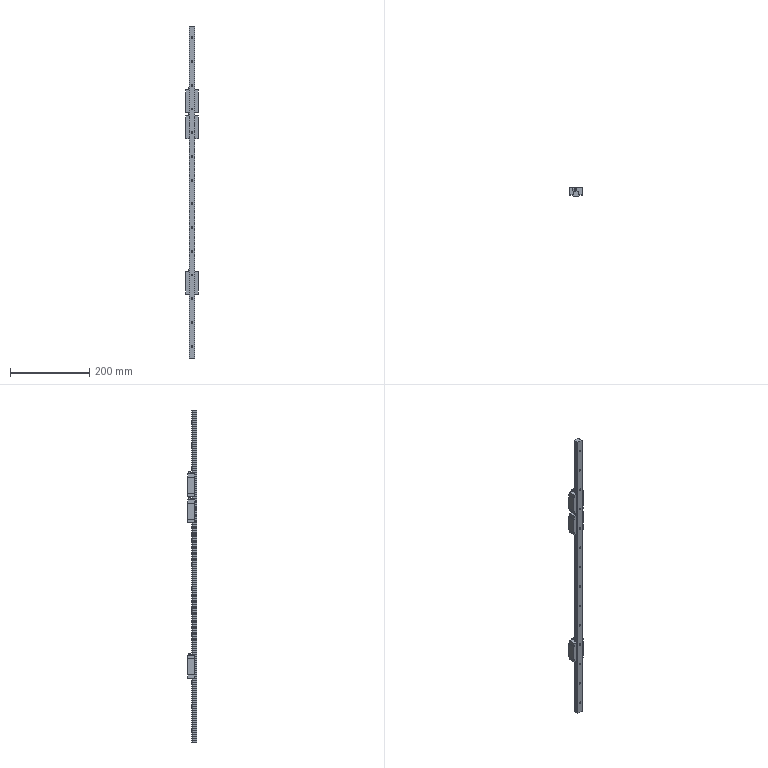Part | NX | features BREP 4 | 4 solids | 236 faces | box 34 x 24 x 840 mm | volume 231169 mm3 | plane 114 | cylinder 92 | cone 24 | torus 6 | commonest cylinder face diameters 4.5 x40 8.1 x28 3.3 x24